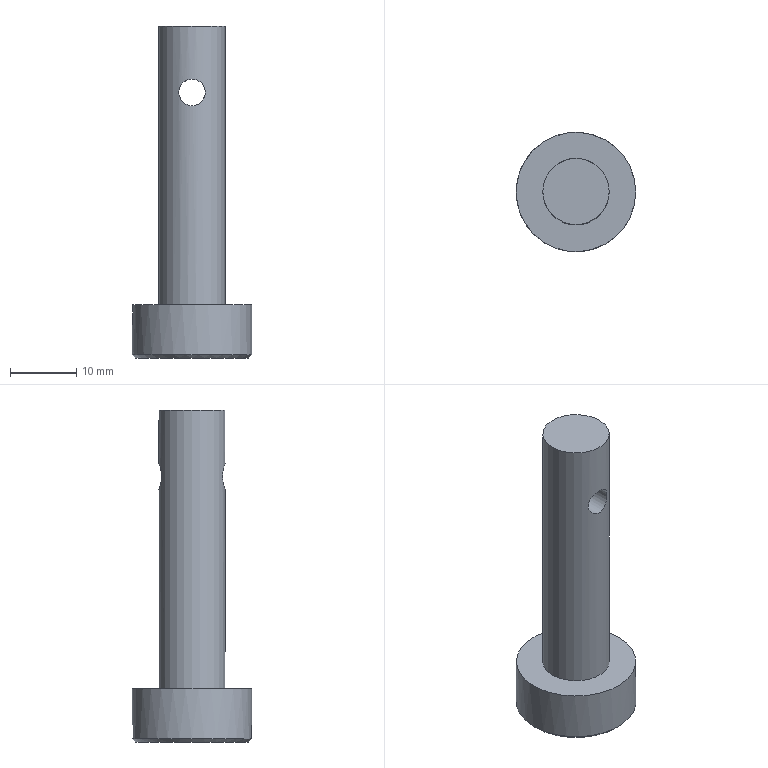Part | NX | features CYLINDER 2, DATUM_CSYS 2, CHAMFER 1, EXTRUDE 1, SKETCH 1 | 1 solid | 7 faces | box 18 x 18 x 50 mm | volume 5204 mm3 | cylinder 3 | plane 3 | cone 1 | commonest cylinder face diameters 4 x1 10 x1 18 x1
STEP:
#1=CARTESIAN_POINT('',(5.,0.,50.));
#2=VERTEX_POINT('',#1);
#3=CARTESIAN_POINT('',(0.,0.,50.));
#4=DIRECTION('',(0.,0.,-1.));
#5=DIRECTION('',(1.,0.,0.));
#6=AXIS2_PLACEMENT_3D('',#3,#4,#5);
#7=CIRCLE('',#6,5.);
#8=EDGE_CURVE('',#2,#2,#7,.T.);
#9=ORIENTED_EDGE('',*,*,#8,.T.);
#10=EDGE_LOOP('',(#9));
#11=FACE_BOUND('',#10,.T.);
#12=CARTESIAN_POINT('',(5.,0.,8.));
#13=VERTEX_POINT('',#12);
#14=CARTESIAN_POINT('',(0.,0.,8.));
#15=DIRECTION('',(0.,0.,1.));
#16=DIRECTION('',(1.,0.,0.));
#17=AXIS2_PLACEMENT_3D('',#14,#15,#16);
#18=CIRCLE('',#17,5.);
#19=EDGE_CURVE('',#13,#13,#18,.T.);
#20=ORIENTED_EDGE('',*,*,#19,.T.);
#21=EDGE_LOOP('',(#20));
#22=FACE_BOUND('',#21,.T.);
#23=CARTESIAN_POINT('',(0.,5.,42.));
#24=VERTEX_POINT('',#23);
#25=CARTESIAN_POINT('',(1.569,4.8,41.566));
#26=CARTESIAN_POINT('',(-0.000227,5.1,42.217));
#27=CARTESIAN_POINT('',(-1.568,4.8,41.565));
#28=CARTESIAN_POINT('',(-2.216,4.474,40.004));
#29=CARTESIAN_POINT('',(-1.567,4.8,38.433));
#30=CARTESIAN_POINT('',(-0.003317,5.1,37.784));
#31=CARTESIAN_POINT('',(1.568,4.8,38.433));
#32=CARTESIAN_POINT('',(2.216,4.474,39.998));
#33=CARTESIAN_POINT('',(1.569,4.8,41.566));
#34=CARTESIAN_POINT('',(-0.000227,5.1,42.217));
#35=CARTESIAN_POINT('',(-1.568,4.8,41.565));
#36=B_SPLINE_CURVE_WITH_KNOTS('',3,(#25,#26,#27,#28,#29,#30,#31,#32,#33,#34,#35),.UNSPECIFIED.,.T.,.F.,(1,1,1,1,1,1,1,1,1,1,1,1,1,1,1),(-0.004738,-0.003159,-0.001579,0.,0.001579,0.003159,0.004738,0.006318,0.007897,0.009477,0.01106,0.01264,0.01421,0.01579,0.01737),.UNSPECIFIED.);
#37=EDGE_CURVE('',#24,#24,#36,.T.);
#38=ORIENTED_EDGE('',*,*,#37,.T.);
#39=EDGE_LOOP('',(#38));
#40=FACE_BOUND('',#39,.T.);
#41=CARTESIAN_POINT('',(0.,-5.,42.));
#42=VERTEX_POINT('',#41);
#43=CARTESIAN_POINT('',(-1.569,-4.8,41.566));
#44=CARTESIAN_POINT('',(0.000227,-5.1,42.217));
#45=CARTESIAN_POINT('',(1.568,-4.8,41.565));
#46=CARTESIAN_POINT('',(2.216,-4.474,40.004));
#47=CARTESIAN_POINT('',(1.567,-4.8,38.433));
#48=CARTESIAN_POINT('',(0.003317,-5.1,37.784));
#49=CARTESIAN_POINT('',(-1.568,-4.8,38.433));
#50=CARTESIAN_POINT('',(-2.216,-4.474,39.998));
#51=CARTESIAN_POINT('',(-1.569,-4.8,41.566));
#52=CARTESIAN_POINT('',(0.000227,-5.1,42.217));
#53=CARTESIAN_POINT('',(1.568,-4.8,41.565));
#54=B_SPLINE_CURVE_WITH_KNOTS('',3,(#43,#44,#45,#46,#47,#48,#49,#50,#51,#52,#53),.UNSPECIFIED.,.T.,.F.,(1,1,1,1,1,1,1,1,1,1,1,1,1,1,1),(-0.004738,-0.003159,-0.001579,0.,0.001579,0.003159,0.004738,0.006318,0.007897,0.009477,0.01106,0.01264,0.01421,0.01579,0.01737),.UNSPECIFIED.);
#55=EDGE_CURVE('',#42,#42,#54,.T.);
#56=ORIENTED_EDGE('',*,*,#55,.T.);
#57=EDGE_LOOP('',(#56));
#58=FACE_BOUND('',#57,.T.);
#59=CARTESIAN_POINT('',(0.,0.,8.));
#60=DIRECTION('',(0.,0.,1.));
#61=DIRECTION('',(1.,0.,0.));
#62=AXIS2_PLACEMENT_3D('',#59,#60,#61);
#63=CYLINDRICAL_SURFACE('',#62,5.);
#64=ADVANCED_FACE('',(#11,#22,#40,#58),#63,.T.);
#65=ORIENTED_EDGE('',*,*,#19,.F.);
#66=EDGE_LOOP('',(#65));
#67=FACE_BOUND('',#66,.T.);
#68=CARTESIAN_POINT('',(9.,0.,8.));
#69=VERTEX_POINT('',#68);
#70=CARTESIAN_POINT('',(0.,0.,8.));
#71=DIRECTION('',(0.,0.,-1.));
#72=DIRECTION('',(1.,0.,0.));
#73=AXIS2_PLACEMENT_3D('',#70,#71,#72);
#74=CIRCLE('',#73,9.);
#75=EDGE_CURVE('',#69,#69,#74,.T.);
#76=ORIENTED_EDGE('',*,*,#75,.F.);
#77=EDGE_LOOP('',(#76));
#78=FACE_BOUND('',#77,.T.);
#79=CARTESIAN_POINT('',(0.,0.,8.));
#80=DIRECTION('',(0.,0.,1.));
#81=DIRECTION('',(1.,0.,0.));
#82=AXIS2_PLACEMENT_3D('',#79,#80,#81);
#83=PLANE('',#82);
#84=ADVANCED_FACE('',(#67,#78),#83,.T.);
#85=CARTESIAN_POINT('',(-8.5,0.,0.));
#86=VERTEX_POINT('',#85);
#87=CARTESIAN_POINT('',(0.,0.,0.));
#88=DIRECTION('',(0.,0.,-1.));
#89=DIRECTION('',(-1.,0.,0.));
#90=AXIS2_PLACEMENT_3D('',#87,#88,#89);
#91=CIRCLE('',#90,8.5);
#92=EDGE_CURVE('',#86,#86,#91,.T.);
#93=ORIENTED_EDGE('',*,*,#92,.T.);
#94=EDGE_LOOP('',(#93));
#95=FACE_BOUND('',#94,.T.);
#96=CARTESIAN_POINT('',(0.,0.,0.));
#97=DIRECTION('',(0.,0.,-1.));
#98=DIRECTION('',(-1.,0.,0.));
#99=AXIS2_PLACEMENT_3D('',#96,#97,#98);
#100=PLANE('',#99);
#101=ADVANCED_FACE('',(#95),#100,.T.);
#102=CARTESIAN_POINT('',(-9.,0.,0.5));
#103=VERTEX_POINT('',#102);
#104=CARTESIAN_POINT('',(0.,0.,0.5));
#105=DIRECTION('',(0.,0.,-1.));
#106=DIRECTION('',(-1.,0.,0.));
#107=AXIS2_PLACEMENT_3D('',#104,#105,#106);
#108=CIRCLE('',#107,9.);
#109=EDGE_CURVE('',#103,#103,#108,.F.);
#110=ORIENTED_EDGE('',*,*,#109,.T.);
#111=EDGE_LOOP('',(#110));
#112=FACE_BOUND('',#111,.T.);
#113=ORIENTED_EDGE('',*,*,#75,.T.);
#114=EDGE_LOOP('',(#113));
#115=FACE_BOUND('',#114,.T.);
#116=CARTESIAN_POINT('',(0.,0.,0.));
#117=DIRECTION('',(0.,0.,1.));
#118=DIRECTION('',(1.,0.,0.));
#119=AXIS2_PLACEMENT_3D('',#116,#117,#118);
#120=CYLINDRICAL_SURFACE('',#119,9.);
#121=ADVANCED_FACE('',(#112,#115),#120,.T.);
#122=ORIENTED_EDGE('',*,*,#8,.F.);
#123=EDGE_LOOP('',(#122));
#124=FACE_BOUND('',#123,.T.);
#125=CARTESIAN_POINT('',(0.,0.,50.));
#126=DIRECTION('',(0.,0.,1.));
#127=DIRECTION('',(1.,0.,0.));
#128=AXIS2_PLACEMENT_3D('',#125,#126,#127);
#129=PLANE('',#128);
#130=ADVANCED_FACE('',(#124),#129,.T.);
#131=ORIENTED_EDGE('',*,*,#55,.F.);
#132=EDGE_LOOP('',(#131));
#133=FACE_BOUND('',#132,.T.);
#134=ORIENTED_EDGE('',*,*,#37,.F.);
#135=EDGE_LOOP('',(#134));
#136=FACE_BOUND('',#135,.T.);
#137=CARTESIAN_POINT('',(0.,-5.,40.));
#138=DIRECTION('',(0.,1.,0.));
#139=DIRECTION('',(0.,0.,1.));
#140=AXIS2_PLACEMENT_3D('',#137,#138,#139);
#141=CYLINDRICAL_SURFACE('',#140,2.);
#142=ADVANCED_FACE('',(#133,#136),#141,.F.);
#143=ORIENTED_EDGE('',*,*,#92,.F.);
#144=EDGE_LOOP('',(#143));
#145=FACE_BOUND('',#144,.T.);
#146=ORIENTED_EDGE('',*,*,#109,.F.);
#147=EDGE_LOOP('',(#146));
#148=FACE_BOUND('',#147,.T.);
#149=CARTESIAN_POINT('',(0.,0.,0.5));
#150=DIRECTION('',(0.,0.,1.));
#151=DIRECTION('',(1.,0.,0.));
#152=AXIS2_PLACEMENT_3D('',#149,#150,#151);
#153=CONICAL_SURFACE('',#152,9.,0.7854);
#154=ADVANCED_FACE('',(#145,#148),#153,.T.);
#155=CLOSED_SHELL('',(#64,#84,#101,#121,#130,#142,#154));
#156=MANIFOLD_SOLID_BREP('',#155);
#157=(LENGTH_UNIT()NAMED_UNIT(*)SI_UNIT(.MILLI.,.METRE.));
#158=UNCERTAINTY_MEASURE_WITH_UNIT(LENGTH_MEASURE(0.0508),#157,'','');
#159=(NAMED_UNIT(*)PLANE_ANGLE_UNIT()SI_UNIT($,.RADIAN.));
#160=(NAMED_UNIT(*)SI_UNIT($,.STERADIAN.)SOLID_ANGLE_UNIT());
#161=(GEOMETRIC_REPRESENTATION_CONTEXT(3)GLOBAL_UNCERTAINTY_ASSIGNED_CONTEXT((#158))GLOBAL_UNIT_ASSIGNED_CONTEXT((#157,#159,#160))REPRESENTATION_CONTEXT('',''));
#162=ADVANCED_BREP_SHAPE_REPRESENTATION('',(#156),#161);